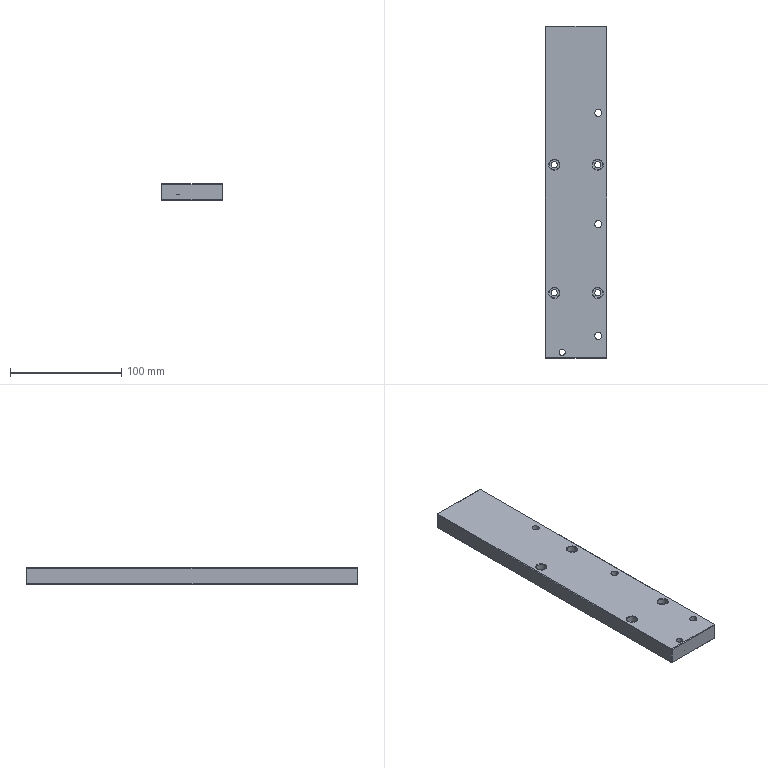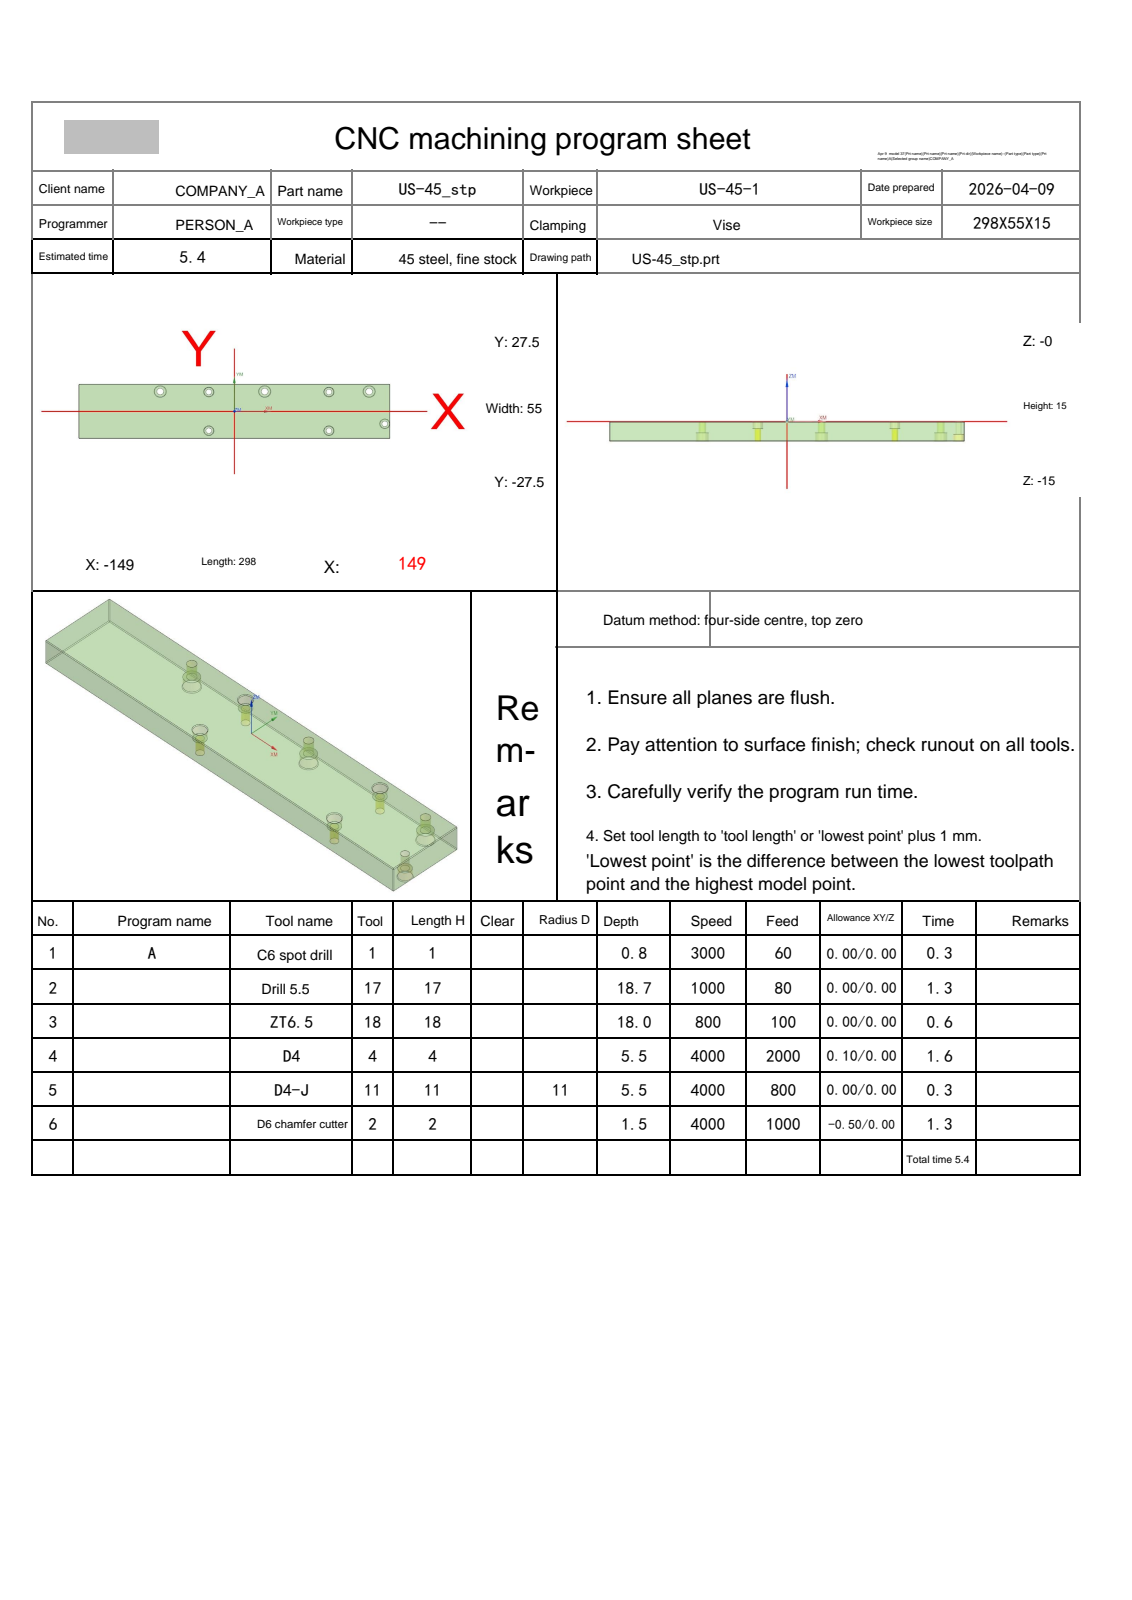NC program | NX | posted by the shop | part box 55 x 298 x 15 mm
Whole program:
%
O0001
(Machine time: 6.47 MIN)
(===Total Tool:6===)
(T1=C6 spot drill   D=6.   R=0.   D-  H01 Z=-0.8  )
(T17=drill 5.5  D=5.5  DR_a=118 D-  H17 Z=-18.65)
(T18=ZT6.5  D=6.5  DR_a=118 D-  H18 Z=-18.  )
(T4=D4      D=4.   R=0.   D-  H04 Z=-5.5  )
(T11=D4-J   D=4.   R=0.   D11 H11 Z=-5.5  )
(T2=D6 chamfer cutter   D=6.   R=0.   D-  H02 Z=-1.5  )
G80 G90 G17 G49 G40
G91 G28 Z0
M01
N1 T01 M06
(C6 spot drill  D=6. R=0. H=01 ce=0.00 di=0.00)
G00 G90 G54 X-71. Y20. M03 S3000
G43 H01 Z20.
M08
G98 G81 X-71. Y20. Z-.8 R1. F60.
X-24.5 Y19.5
Y-19.5
X29. Y20.
X90.5 Y-19.5
Y19.5
X129. Y20.
X144. Y-12.5
G80
G00 Z20.
G91 G28 Z0.0
M05
M09
G91 G28 Z0.0
M01
N2 T17 M06
(drill 5.5 D=5.5 DR_a=118 H=17)
G00 G90 G54 X144. Y-12.5 M03 S1000
G43 H17 Z20.
M08
G98 G83 X144. Y-12.5 Z-18. R1. F80. Q1.
G80
G00 Z20.
G00 G90 X90.5 Y-19.5 M03 S1000
Z20.
G98 G83 X90.5 Y-19.5 Z-18.652 R1. F80. Q1.
Y19.5
X-24.5
Y-19.5
G80
G00 Z20.
G91 G28 Z0.0
M05
M09
G91 G28 Z0.0
M01
N3 T18 M06
(ZT6.5 D=6.5 DR_a=118 H=18)
G00 G90 G54 X-71. Y20. M03 S800
G43 H18 Z20.
M08
G98 G83 X-71. Y20. Z-18. R1. F100. Q1.
X29.
X129.
G80
G00 Z20.
G91 G28 Z0.0
M05
M09
G91 G28 Z0.0
M01
N4 T04 M06
(D4  D=4. R=0. H=04 ce=0.10 di=0.00)
G00 G90 G54 X90.5 Y-19.5 M03 S4000
G43 H04 Z20.
M08
Z1.
G03 X91.1 Y-18.9 I0.0 J.6 F2000.
X90.5 Y-18.3 I-.6 J0.0
X90.5 Y-18.3 Z.8 I0.0 J-1.2
X90.5 Y-18.3 Z.6 I0.0 J-1.2
X90.5 Y-18.3 Z.4 I0.0 J-1.2
X90.5 Y-18.3 Z.2 I0.0 J-1.2
X90.5 Y-18.3 Z0.0 I0.0 J-1.2
X90.5 Y-18.3 Z-.2 I0.0 J-1.2
X90.5 Y-18.3 Z-.4 I0.0 J-1.2
X90.5 Y-18.3 Z-.6 I0.0 J-1.2
X90.5 Y-18.3 Z-.8 I0.0 J-1.2
X90.5 Y-18.3 Z-1. I0.0 J-1.2
X90.5 Y-18.3 Z-1.2 I0.0 J-1.2
X90.5 Y-18.3 Z-1.4 I0.0 J-1.2
X90.5 Y-18.3 Z-1.6 I0.0 J-1.2
X90.5 Y-18.3 Z-1.8 I0.0 J-1.2
X90.5 Y-18.3 Z-2. I0.0 J-1.2
X90.5 Y-18.3 Z-2.2 I0.0 J-1.2
X90.5 Y-18.3 Z-2.4 I0.0 J-1.2
X90.5 Y-18.3 Z-2.6 I0.0 J-1.2
X90.5 Y-18.3 Z-2.8 I0.0 J-1.2
X90.5 Y-18.3 Z-3. I0.0 J-1.2
X90.5 Y-18.3 Z-3.2 I0.0 J-1.2
X90.5 Y-18.3 Z-3.4 I0.0 J-1.2
X90.5 Y-18.3 Z-3.6 I0.0 J-1.2
X90.5 Y-18.3 Z-3.8 I0.0 J-1.2
X90.5 Y-18.3 Z-4. I0.0 J-1.2
X90.5 Y-18.3 Z-4.2 I0.0 J-1.2
X90.5 Y-18.3 Z-4.4 I0.0 J-1.2
X90.5 Y-18.3 Z-4.6 I0.0 J-1.2
X90.5 Y-18.3 Z-4.8 I0.0 J-1.2
X90.5 Y-18.3 Z-5. I0.0 J-1.2
X90.5 Y-18.3 Z-5.2 I0.0 J-1.2
X90.5 Y-18.3 Z-5.4 I0.0 J-1.2
X90.501 Y-20.7 Z-5.5 I0.0 J-1.2
X91.7 Y-19.5 I-.001 J1.2
X90.5 Y-18.3 I-1.2 J0.0
X89.3 Y-19.5 I0.0 J-1.2
X90.5 Y-20.7 I1.2 J0.0
X91.1 Y-20.1 I0.0 J.6
X90.5 Y-19.5 I-.6 J0.0
G00 Z1.
G03 X91.7 Y-18.3 I0.0 J1.2
X90.5 Y-17.1 I-1.2 J0.0
X90.5 Y-17.1 Z.8 I0.0 J-2.4
X90.5 Y-17.1 Z.6 I0.0 J-2.4
X90.5 Y-17.1 Z.4 I0.0 J-2.4
X90.5 Y-17.1 Z.2 I0.0 J-2.4
X90.5 Y-17.1 Z0.0 I0.0 J-2.4
X90.5 Y-17.1 Z-.2 I0.0 J-2.4
X90.5 Y-17.1 Z-.4 I0.0 J-2.4
X90.5 Y-17.1 Z-.6 I0.0 J-2.4
X90.5 Y-17.1 Z-.8 I0.0 J-2.4
X90.5 Y-17.1 Z-1. I0.0 J-2.4
X90.5 Y-17.1 Z-1.2 I0.0 J-2.4
X90.5 Y-17.1 Z-1.4 I0.0 J-2.4
X90.5 Y-17.1 Z-1.6 I0.0 J-2.4
X90.5 Y-17.1 Z-1.8 I0.0 J-2.4
X90.5 Y-17.1 Z-2. I0.0 J-2.4
X90.5 Y-17.1 Z-2.2 I0.0 J-2.4
X90.5 Y-17.1 Z-2.4 I0.0 J-2.4
X90.5 Y-17.1 Z-2.6 I0.0 J-2.4
X90.5 Y-17.1 Z-2.8 I0.0 J-2.4
X90.5 Y-17.1 Z-3. I0.0 J-2.4
X90.5 Y-17.1 Z-3.2 I0.0 J-2.4
X90.5 Y-17.1 Z-3.4 I0.0 J-2.4
X90.5 Y-17.1 Z-3.6 I0.0 J-2.4
X90.5 Y-17.1 Z-3.8 I0.0 J-2.4
X90.5 Y-17.1 Z-4. I0.0 J-2.4
X90.5 Y-17.1 Z-4.2 I0.0 J-2.4
X90.5 Y-17.1 Z-4.4 I0.0 J-2.4
X90.5 Y-17.1 Z-4.6 I0.0 J-2.4
X90.5 Y-17.1 Z-4.8 I0.0 J-2.4
X90.5 Y-17.1 Z-5. I0.0 J-2.4
X90.5 Y-17.1 Z-5.2 I0.0 J-2.4
X90.5 Y-17.1 Z-5.4 I0.0 J-2.4
X90.501 Y-21.9 Z-5.5 I0.0 J-2.4
X92.9 Y-19.5 I-.001 J2.4
X90.5 Y-17.1 I-2.4 J0.0
X88.1 Y-19.5 I0.0 J-2.4
X90.5 Y-21.9 I2.4 J0.0
G01 X90.501
G03 X91.701 Y-20.7 I-.001 J1.2
X90.501 Y-19.5 I-1.2 J0.0
G00 Z20.
X90.5 Y19.5
Z1.
G03 X91.1 Y20.1 I0.0 J.6
X90.5 Y20.7 I-.6 J0.0
X90.5 Y20.7 Z.8 I0.0 J-1.2
X90.5 Y20.7 Z.6 I0.0 J-1.2
X90.5 Y20.7 Z.4 I0.0 J-1.2
X90.5 Y20.7 Z.2 I0.0 J-1.2
X90.5 Y20.7 Z0.0 I0.0 J-1.2
X90.5 Y20.7 Z-.2 I0.0 J-1.2
X90.5 Y20.7 Z-.4 I0.0 J-1.2
X90.5 Y20.7 Z-.6 I0.0 J-1.2
X90.5 Y20.7 Z-.8 I0.0 J-1.2
X90.5 Y20.7 Z-1. I0.0 J-1.2
X90.5 Y20.7 Z-1.2 I0.0 J-1.2
X90.5 Y20.7 Z-1.4 I0.0 J-1.2
X90.5 Y20.7 Z-1.6 I0.0 J-1.2
X90.5 Y20.7 Z-1.8 I0.0 J-1.2
X90.5 Y20.7 Z-2. I0.0 J-1.2
X90.5 Y20.7 Z-2.2 I0.0 J-1.2
X90.5 Y20.7 Z-2.4 I0.0 J-1.2
X90.5 Y20.7 Z-2.6 I0.0 J-1.2
X90.5 Y20.7 Z-2.8 I0.0 J-1.2
X90.5 Y20.7 Z-3. I0.0 J-1.2
X90.5 Y20.7 Z-3.2 I0.0 J-1.2
X90.5 Y20.7 Z-3.4 I0.0 J-1.2
X90.5 Y20.7 Z-3.6 I0.0 J-1.2
X90.5 Y20.7 Z-3.8 I0.0 J-1.2
X90.5 Y20.7 Z-4. I0.0 J-1.2
X90.5 Y20.7 Z-4.2 I0.0 J-1.2
X90.5 Y20.7 Z-4.4 I0.0 J-1.2
X90.5 Y20.7 Z-4.6 I0.0 J-1.2
X90.5 Y20.7 Z-4.8 I0.0 J-1.2
X90.5 Y20.7 Z-5. I0.0 J-1.2
X90.5 Y20.7 Z-5.2 I0.0 J-1.2
X90.5 Y20.7 Z-5.4 I0.0 J-1.2
X90.501 Y18.3 Z-5.5 I0.0 J-1.2
X91.7 Y19.5 I-.001 J1.2
X90.5 Y20.7 I-1.2 J0.0
X89.3 Y19.5 I0.0 J-1.2
X90.5 Y18.3 I1.2 J0.0
X91.1 Y18.9 I0.0 J.6
X90.5 Y19.5 I-.6 J0.0
G00 Z1.
G03 X91.7 Y20.7 I0.0 J1.2
X90.5 Y21.9 I-1.2 J0.0
X90.5 Y21.9 Z.8 I0.0 J-2.4
X90.5 Y21.9 Z.6 I0.0 J-2.4
X90.5 Y21.9 Z.4 I0.0 J-2.4
X90.5 Y21.9 Z.2 I0.0 J-2.4
X90.5 Y21.9 Z0.0 I0.0 J-2.4
X90.5 Y21.9 Z-.2 I0.0 J-2.4
X90.5 Y21.9 Z-.4 I0.0 J-2.4
X90.5 Y21.9 Z-.6 I0.0 J-2.4
X90.5 Y21.9 Z-.8 I0.0 J-2.4
X90.5 Y21.9 Z-1. I0.0 J-2.4
X90.5 Y21.9 Z-1.2 I0.0 J-2.4
X90.5 Y21.9 Z-1.4 I0.0 J-2.4
X90.5 Y21.9 Z-1.6 I0.0 J-2.4
X90.5 Y21.9 Z-1.8 I0.0 J-2.4
X90.5 Y21.9 Z-2. I0.0 J-2.4
X90.5 Y21.9 Z-2.2 I0.0 J-2.4
X90.5 Y21.9 Z-2.4 I0.0 J-2.4
X90.5 Y21.9 Z-2.6 I0.0 J-2.4
X90.5 Y21.9 Z-2.8 I0.0 J-2.4
X90.5 Y21.9 Z-3. I0.0 J-2.4
X90.5 Y21.9 Z-3.2 I0.0 J-2.4
X90.5 Y21.9 Z-3.4 I0.0 J-2.4
X90.5 Y21.9 Z-3.6 I0.0 J-2.4
X90.5 Y21.9 Z-3.8 I0.0 J-2.4
X90.5 Y21.9 Z-4. I0.0 J-2.4
X90.5 Y21.9 Z-4.2 I0.0 J-2.4
X90.5 Y21.9 Z-4.4 I0.0 J-2.4
X90.5 Y21.9 Z-4.6 I0.0 J-2.4
X90.5 Y21.9 Z-4.8 I0.0 J-2.4
X90.5 Y21.9 Z-5. I0.0 J-2.4
X90.5 Y21.9 Z-5.2 I0.0 J-2.4
X90.5 Y21.9 Z-5.4 I0.0 J-2.4
X90.501 Y17.1 Z-5.5 I0.0 J-2.4
X92.9 Y19.5 I-.001 J2.4
X90.5 Y21.9 I-2.4 J0.0
X88.1 Y19.5 I0.0 J-2.4
X90.5 Y17.1 I2.4 J0.0
G01 X90.501
G03 X91.701 Y18.3 I-.001 J1.2
X90.501 Y19.5 I-1.2 J0.0
G00 Z20.
X-24.5
Z1.
G03 X-23.9 Y20.1 I0.0 J.6
X-24.5 Y20.7 I-.6 J0.0
X-24.5 Y20.7 Z.8 I0.0 J-1.2
X-24.5 Y20.7 Z.6 I0.0 J-1.2
X-24.5 Y20.7 Z.4 I0.0 J-1.2
X-24.5 Y20.7 Z.2 I0.0 J-1.2
X-24.5 Y20.7 Z0.0 I0.0 J-1.2
X-24.5 Y20.7 Z-.2 I0.0 J-1.2
X-24.5 Y20.7 Z-.4 I0.0 J-1.2
X-24.5 Y20.7 Z-.6 I0.0 J-1.2
X-24.5 Y20.7 Z-.8 I0.0 J-1.2
X-24.5 Y20.7 Z-1. I0.0 J-1.2
X-24.5 Y20.7 Z-1.2 I0.0 J-1.2
X-24.5 Y20.7 Z-1.4 I0.0 J-1.2
X-24.5 Y20.7 Z-1.6 I0.0 J-1.2
X-24.5 Y20.7 Z-1.8 I0.0 J-1.2
X-24.5 Y20.7 Z-2. I0.0 J-1.2
X-24.5 Y20.7 Z-2.2 I0.0 J-1.2
X-24.5 Y20.7 Z-2.4 I0.0 J-1.2
X-24.5 Y20.7 Z-2.6 I0.0 J-1.2
X-24.5 Y20.7 Z-2.8 I0.0 J-1.2
X-24.5 Y20.7 Z-3. I0.0 J-1.2
X-24.5 Y20.7 Z-3.2 I0.0 J-1.2
X-24.5 Y20.7 Z-3.4 I0.0 J-1.2
X-24.5 Y20.7 Z-3.6 I0.0 J-1.2
X-24.5 Y20.7 Z-3.8 I0.0 J-1.2
X-24.5 Y20.7 Z-4. I0.0 J-1.2
X-24.5 Y20.7 Z-4.2 I0.0 J-1.2
X-24.5 Y20.7 Z-4.4 I0.0 J-1.2
X-24.5 Y20.7 Z-4.6 I0.0 J-1.2
X-24.5 Y20.7 Z-4.8 I0.0 J-1.2
X-24.5 Y20.7 Z-5. I0.0 J-1.2
X-24.5 Y20.7 Z-5.2 I0.0 J-1.2
X-24.5 Y20.7 Z-5.4 I0.0 J-1.2
X-24.499 Y18.3 Z-5.5 I0.0 J-1.2
X-23.3 Y19.5 I-.001 J1.2
X-24.5 Y20.7 I-1.2 J0.0
X-25.7 Y19.5 I0.0 J-1.2
X-24.5 Y18.3 I1.2 J0.0
X-23.9 Y18.9 I0.0 J.6
X-24.5 Y19.5 I-.6 J0.0
G00 Z1.
G03 X-23.3 Y20.7 I0.0 J1.2
X-24.5 Y21.9 I-1.2 J0.0
X-24.5 Y21.9 Z.8 I0.0 J-2.4
X-24.5 Y21.9 Z.6 I0.0 J-2.4
X-24.5 Y21.9 Z.4 I0.0 J-2.4
X-24.5 Y21.9 Z.2 I0.0 J-2.4
X-24.5 Y21.9 Z0.0 I0.0 J-2.4
X-24.5 Y21.9 Z-.2 I0.0 J-2.4
X-24.5 Y21.9 Z-.4 I0.0 J-2.4
X-24.5 Y21.9 Z-.6 I0.0 J-2.4
X-24.5 Y21.9 Z-.8 I0.0 J-2.4
X-24.5 Y21.9 Z-1. I0.0 J-2.4
X-24.5 Y21.9 Z-1.2 I0.0 J-2.4
X-24.5 Y21.9 Z-1.4 I0.0 J-2.4
X-24.5 Y21.9 Z-1.6 I0.0 J-2.4
X-24.5 Y21.9 Z-1.8 I0.0 J-2.4
X-24.5 Y21.9 Z-2. I0.0 J-2.4
X-24.5 Y21.9 Z-2.2 I0.0 J-2.4
X-24.5 Y21.9 Z-2.4 I0.0 J-2.4
X-24.5 Y21.9 Z-2.6 I0.0 J-2.4
X-24.5 Y21.9 Z-2.8 I0.0 J-2.4
X-24.5 Y21.9 Z-3. I0.0 J-2.4
X-24.5 Y21.9 Z-3.2 I0.0 J-2.4
X-24.5 Y21.9 Z-3.4 I0.0 J-2.4
X-24.5 Y21.9 Z-3.6 I0.0 J-2.4
X-24.5 Y21.9 Z-3.8 I0.0 J-2.4
X-24.5 Y21.9 Z-4. I0.0 J-2.4
X-24.5 Y21.9 Z-4.2 I0.0 J-2.4
X-24.5 Y21.9 Z-4.4 I0.0 J-2.4
X-24.5 Y21.9 Z-4.6 I0.0 J-2.4
X-24.5 Y21.9 Z-4.8 I0.0 J-2.4
X-24.5 Y21.9 Z-5. I0.0 J-2.4
X-24.5 Y21.9 Z-5.2 I0.0 J-2.4
X-24.5 Y21.9 Z-5.4 I0.0 J-2.4
X-24.499 Y17.1 Z-5.5 I0.0 J-2.4
X-22.1 Y19.5 I-.001 J2.4
X-24.5 Y21.9 I-2.4 J0.0
X-26.9 Y19.5 I0.0 J-2.4
X-24.5 Y17.1 I2.4 J0.0
G01 X-24.499
G03 X-23.299 Y18.3 I-.001 J1.2
X-24.499 Y19.5 I-1.2 J0.0
G00 Z20.
X-24.5 Y-19.5
Z1.
G03 X-23.9 Y-18.9 I0.0 J.6
X-24.5 Y-18.3 I-.6 J0.0
X-24.5 Y-18.3 Z.8 I0.0 J-1.2
X-24.5 Y-18.3 Z.6 I0.0 J-1.2
X-24.5 Y-18.3 Z.4 I0.0 J-1.2
X-24.5 Y-18.3 Z.2 I0.0 J-1.2
X-24.5 Y-18.3 Z0.0 I0.0 J-1.2
X-24.5 Y-18.3 Z-.2 I0.0 J-1.2
X-24.5 Y-18.3 Z-.4 I0.0 J-1.2
X-24.5 Y-18.3 Z-.6 I0.0 J-1.2
X-24.5 Y-18.3 Z-.8 I0.0 J-1.2
X-24.5 Y-18.3 Z-1. I0.0 J-1.2
X-24.5 Y-18.3 Z-1.2 I0.0 J-1.2
X-24.5 Y-18.3 Z-1.4 I0.0 J-1.2
X-24.5 Y-18.3 Z-1.6 I0.0 J-1.2
X-24.5 Y-18.3 Z-1.8 I0.0 J-1.2
X-24.5 Y-18.3 Z-2. I0.0 J-1.2
X-24.5 Y-18.3 Z-2.2 I0.0 J-1.2
X-24.5 Y-18.3 Z-2.4 I0.0 J-1.2
X-24.5 Y-18.3 Z-2.6 I0.0 J-1.2
X-24.5 Y-18.3 Z-2.8 I0.0 J-1.2
X-24.5 Y-18.3 Z-3. I0.0 J-1.2
X-24.5 Y-18.3 Z-3.2 I0.0 J-1.2
X-24.5 Y-18.3 Z-3.4 I0.0 J-1.2
X-24.5 Y-18.3 Z-3.6 I0.0 J-1.2
X-24.5 Y-18.3 Z-3.8 I0.0 J-1.2
X-24.5 Y-18.3 Z-4. I0.0 J-1.2
X-24.5 Y-18.3 Z-4.2 I0.0 J-1.2
X-24.5 Y-18.3 Z-4.4 I0.0 J-1.2
X-24.5 Y-18.3 Z-4.6 I0.0 J-1.2
X-24.5 Y-18.3 Z-4.8 I0.0 J-1.2
X-24.5 Y-18.3 Z-5. I0.0 J-1.2
X-24.5 Y-18.3 Z-5.2 I0.0 J-1.2
X-24.5 Y-18.3 Z-5.4 I0.0 J-1.2
X-24.499 Y-20.7 Z-5.5 I0.0 J-1.2
X-23.3 Y-19.5 I-.001 J1.2
X-24.5 Y-18.3 I-1.2 J0.0
X-25.7 Y-19.5 I0.0 J-1.2
X-24.5 Y-20.7 I1.2 J0.0
X-23.9 Y-20.1 I0.0 J.6
X-24.5 Y-19.5 I-.6 J0.0
G00 Z1.
G03 X-23.3 Y-18.3 I0.0 J1.2
X-24.5 Y-17.1 I-1.2 J0.0
X-24.5 Y-17.1 Z.8 I0.0 J-2.4
X-24.5 Y-17.1 Z.6 I0.0 J-2.4
X-24.5 Y-17.1 Z.4 I0.0 J-2.4
X-24.5 Y-17.1 Z.2 I0.0 J-2.4
X-24.5 Y-17.1 Z0.0 I0.0 J-2.4
X-24.5 Y-17.1 Z-.2 I0.0 J-2.4
X-24.5 Y-17.1 Z-.4 I0.0 J-2.4
X-24.5 Y-17.1 Z-.6 I0.0 J-2.4
X-24.5 Y-17.1 Z-.8 I0.0 J-2.4
X-24.5 Y-17.1 Z-1. I0.0 J-2.4
X-24.5 Y-17.1 Z-1.2 I0.0 J-2.4
X-24.5 Y-17.1 Z-1.4 I0.0 J-2.4
X-24.5 Y-17.1 Z-1.6 I0.0 J-2.4
X-24.5 Y-17.1 Z-1.8 I0.0 J-2.4
X-24.5 Y-17.1 Z-2. I0.0 J-2.4
X-24.5 Y-17.1 Z-2.2 I0.0 J-2.4
X-24.5 Y-17.1 Z-2.4 I0.0 J-2.4
X-24.5 Y-17.1 Z-2.6 I0.0 J-2.4
X-24.5 Y-17.1 Z-2.8 I0.0 J-2.4
X-24.5 Y-17.1 Z-3. I0.0 J-2.4
X-24.5 Y-17.1 Z-3.2 I0.0 J-2.4
X-24.5 Y-17.1 Z-3.4 I0.0 J-2.4
X-24.5 Y-17.1 Z-3.6 I0.0 J-2.4
X-24.5 Y-17.1 Z-3.8 I0.0 J-2.4
X-24.5 Y-17.1 Z-4. I0.0 J-2.4
X-24.5 Y-17.1 Z-4.2 I0.0 J-2.4
X-24.5 Y-17.1 Z-4.4 I0.0 J-2.4
X-24.5 Y-17.1 Z-4.6 I0.0 J-2.4
X-24.5 Y-17.1 Z-4.8 I0.0 J-2.4
X-24.5 Y-17.1 Z-5. I0.0 J-2.4
X-24.5 Y-17.1 Z-5.2 I0.0 J-2.4
X-24.5 Y-17.1 Z-5.4 I0.0 J-2.4
X-24.499 Y-21.9 Z-5.5 I0.0 J-2.4
X-22.1 Y-19.5 I-.001 J2.4
X-24.5 Y-17.1 I-2.4 J0.0
X-26.9 Y-19.5 I0.0 J-2.4
X-24.5 Y-21.9 I2.4 J0.0
G01 X-24.499
G03 X-23.299 Y-20.7 I-.001 J1.2
X-24.499 Y-19.5 I-1.2 J0.0
G00 Z20.
G91 G28 Z0.0
M05
M09
G91 G28 Z0.0
M01
N5 T11 M06
(D4-J  D=4. R=0. H=11 ce=0.00 di=0.00)
G00 G90 G54 X90.5 Y-19.5 M03 S4000
G43 H11 Z20.
M08
Z1.
G41 D11
G01 X90.697 Y-19.468 F800.
G03 X91.742 Y-18.242 I-.197 J1.226
X90.5 Y-17. I-1.242 J0.0
X90.5 Y-17. Z-4. I0.0 J-2.5
X88.122 Y-20.273 Z-5.5 I0.0 J-2.5
X90.5 Y-22. I2.378 J.773
X93. Y-19.5 I0.0 J2.5
X90.5 Y-17. I-2.5 J0.0
X88. Y-19.5 I0.0 J-2.5
X88.122 Y-20.273 I2.5 J0.0
X89.304 Y-21.131 I1.181 J.384
X90.546 Y-19.889 I0.0 J1.242
G01 X90.531 Y-19.698
G40 X90.5 Y-19.5
G00 Z20.
Y19.5
Z1.
G41 D11
G01 X90.697 Y19.532
G03 X91.742 Y20.758 I-.197 J1.226
X90.5 Y22. I-1.242 J0.0
X90.5 Y22. Z-4. I0.0 J-2.5
X88.122 Y18.727 Z-5.5 I0.0 J-2.5
X90.5 Y17. I2.378 J.773
X93. Y19.5 I0.0 J2.5
X90.5 Y22. I-2.5 J0.0
X88. Y19.5 I0.0 J-2.5
X88.122 Y18.727 I2.5 J0.0
X89.304 Y17.869 I1.181 J.384
X90.546 Y19.111 I0.0 J1.242
G01 X90.531 Y19.302
G40 X90.5 Y19.5
G00 Z20.
X-24.5
Z1.
G41 D11
G01 X-24.303 Y19.532
G03 X-23.258 Y20.758 I-.197 J1.226
X-24.5 Y22. I-1.242 J0.0
X-24.5 Y22. Z-4. I0.0 J-2.5
X-26.878 Y18.727 Z-5.5 I0.0 J-2.5
X-24.5 Y17. I2.378 J.773
X-22. Y19.5 I0.0 J2.5
X-24.5 Y22. I-2.5 J0.0
X-27. Y19.5 I0.0 J-2.5
X-26.878 Y18.727 I2.5 J0.0
X-25.696 Y17.869 I1.181 J.384
X-24.454 Y19.111 I0.0 J1.242
G01 X-24.469 Y19.302
G40 X-24.5 Y19.5
G00 Z20.
Y-19.5
Z1.
G41 D11
G01 X-24.303 Y-19.468
G03 X-23.258 Y-18.242 I-.197 J1.226
X-24.5 Y-17. I-1.242 J0.0
X-24.5 Y-17. Z-4. I0.0 J-2.5
X-26.878 Y-20.273 Z-5.5 I0.0 J-2.5
X-24.5 Y-22. I2.378 J.773
X-22. Y-19.5 I0.0 J2.5
X-24.5 Y-17. I-2.5 J0.0
X-27. Y-19.5 I0.0 J-2.5
X-26.878 Y-20.273 I2.5 J0.0
X-25.696 Y-21.131 I1.181 J.384
X-24.454 Y-19.889 I0.0 J1.242
G01 X-24.469 Y-19.698
G40 X-24.5 Y-19.5
G00 Z20.
G91 G28 Z0.0
M05
M09
G91 G28 Z0.0
M01
N6 T02 M06
(D6 chamfer cutter  D=6. R=0. H=02 ce=-0.30 di=0.00)
G00 G90 G54 X145.118 Y-11.941 M03 S4000
G43 H02 Z20.
M08
Z-.3
G01 Z-.8 F300.
X145.5 Y-11.75
G03 X144. Y-10.25 I-1.5 J0.0
X141.75 Y-12.5 I0.0 J-2.25
X144. Y-14.75 I2.25 J0.0
X146.25 Y-12.5 I0.0 J2.25
X144. Y-10.25 I-2.25 J0.0
X142.5 Y-11.75 I0.0 J-1.5
G01 X142.882 Y-11.941
Z-.3
G00 Z20.
G00 G90 X130.5 Y20.391 M03 S4000
Z20.
Z-.5
G01 Z-1. F400.
Y21.05
G03 X129. Y22.55 I-1.5 J0.0
X126.45 Y20. I0.0 J-2.55
X129. Y17.45 I2.55 J0.0
X131.55 Y20. I0.0 J2.55
X129. Y22.55 I-2.55 J0.0
X127.5 Y21.05 I0.0 J-1.5
G01 Y20.391
Z-.5
G00 Z20.
X30.5
Z-.5
G01 Z-1.
Y21.05
G03 X29. Y22.55 I-1.5 J0.0
X26.45 Y20. I0.0 J-2.55
X29. Y17.45 I2.55 J0.0
X31.55 Y20. I0.0 J2.55
X29. Y22.55 I-2.55 J0.0
X27.5 Y21.05 I0.0 J-1.5
G01 Y20.391
Z-.5
G00 Z20.
X-69.5
Z-.5
G01 Z-1.
Y21.05
G03 X-71. Y22.55 I-1.5 J0.0
X-73.55 Y20. I0.0 J-2.55
X-71. Y17.45 I2.55 J0.0
X-68.45 Y20. I0.0 J2.55
X-71. Y22.55 I-2.55 J0.0
X-72.5 Y21.05 I0.0 J-1.5
G01 Y20.391
Z-.5
G00 Z20.
G00 G90 X90.509 Y15.998 M03 S4000
Z20.
Z2.5
G01 X90.891 Y16.019 Z2.361 F500.
X91.276 Y16.084 Z2.219
X91.653 Y16.192 Z2.076
X92.014 Y16.341 Z1.934
X92.357 Y16.53 Z1.791
X92.677 Y16.755 Z1.649
X92.969 Y17.015 Z1.507
X93.231 Y17.306 Z1.364
X93.459 Y17.624 Z1.222
X93.604 Y17.876 Z1.116
X93.765 Y18.232 Z.974
X93.886 Y18.604 Z.831
X93.965 Y18.987 Z.689
X94.001 Y19.377 Z.547
X93.993 Y19.768 Z.404
X93.941 Y20.156 Z.262
X93.846 Y20.535 Z.119
X93.71 Y20.902 Z-.023
X93.534 Y21.252 Z-.166
X93.319 Y21.579 Z-.308
X93.07 Y21.88 Z-.45
X92.788 Y22.152 Z-.593
X92.478 Y22.391 Z-.735
X92.144 Y22.593 Z-.878
X91.788 Y22.757 Z-1.02
X91.417 Y22.881 Z-1.162
X91.034 Y22.962 Z-1.305
X90.645 Y23. Z-1.447
X90.5 Z-1.5
G03 X87. Y19.5 I0.0 J-3.5
X90.5 Y16. I3.5 J0.0
X94. Y19.5 I0.0 J3.5
X90.5 Y23. I-3.5 J0.0
X90.002 Y22.964 I0.0 J-3.5
G01 Z1.
G00 Z20.
X90.509 Y-23.002
Z2.5
G01 X90.891 Y-22.981 Z2.361
X91.276 Y-22.916 Z2.219
X91.653 Y-22.808 Z2.076
X92.014 Y-22.659 Z1.934
X92.357 Y-22.47 Z1.791
X92.677 Y-22.245 Z1.649
X92.969 Y-21.985 Z1.507
X93.231 Y-21.694 Z1.364
X93.459 Y-21.376 Z1.222
X93.604 Y-21.124 Z1.116
X93.765 Y-20.768 Z.974
X93.886 Y-20.396 Z.831
X93.965 Y-20.013 Z.689
X94.001 Y-19.623 Z.547
X93.993 Y-19.232 Z.404
X93.941 Y-18.844 Z.262
X93.846 Y-18.465 Z.119
X93.71 Y-18.098 Z-.023
X93.534 Y-17.749 Z-.166
X93.319 Y-17.421 Z-.308
X93.07 Y-17.12 Z-.45
X92.788 Y-16.848 Z-.593
X92.478 Y-16.609 Z-.735
X92.144 Y-16.407 Z-.878
X91.788 Y-16.243 Z-1.02
X91.417 Y-16.119 Z-1.162
X91.034 Y-16.038 Z-1.305
X90.645 Y-16. Z-1.447
X90.5 Z-1.5
G03 X87. Y-19.5 I0.0 J-3.5
X90.5 Y-23. I3.5 J0.0
X94. Y-19.5 I0.0 J3.5
X90.5 Y-16. I-3.5 J0.0
X90.002 Y-16.036 I0.0 J-3.5
G01 Z1.
G00 Z20.
X-24.491 Y-23.002
Z2.5
G01 X-24.109 Y-22.981 Z2.361
X-23.724 Y-22.916 Z2.219
X-23.347 Y-22.808 Z2.076
X-22.986 Y-22.659 Z1.934
X-22.643 Y-22.47 Z1.791
X-22.323 Y-22.245 Z1.649
X-22.031 Y-21.985 Z1.507
X-21.769 Y-21.694 Z1.364
X-21.541 Y-21.376 Z1.222
X-21.396 Y-21.124 Z1.116
X-21.235 Y-20.768 Z.974
X-21.114 Y-20.396 Z.831
X-21.035 Y-20.013 Z.689
X-20.999 Y-19.623 Z.547
X-21.007 Y-19.232 Z.404
X-21.059 Y-18.844 Z.262
X-21.154 Y-18.465 Z.119
X-21.29 Y-18.098 Z-.023
X-21.466 Y-17.749 Z-.166
X-21.681 Y-17.421 Z-.308
X-21.93 Y-17.12 Z-.45
X-22.212 Y-16.848 Z-.593
X-22.522 Y-16.609 Z-.735
X-22.856 Y-16.407 Z-.878
X-23.212 Y-16.243 Z-1.02
X-23.583 Y-16.119 Z-1.162
X-23.966 Y-16.038 Z-1.305
X-24.355 Y-16. Z-1.447
X-24.5 Z-1.5
G03 X-28. Y-19.5 I0.0 J-3.5
X-24.5 Y-23. I3.5 J0.0
X-21. Y-19.5 I0.0 J3.5
X-24.5 Y-16. I-3.5 J0.0
X-24.998 Y-16.036 I0.0 J-3.5
G01 Z1.
G00 Z20.
X-24.491 Y15.998
Z2.5
G01 X-24.109 Y16.019 Z2.361
X-23.724 Y16.084 Z2.219
X-23.347 Y16.192 Z2.076
X-22.986 Y16.341 Z1.934
X-22.643 Y16.53 Z1.791
X-22.323 Y16.755 Z1.649
X-22.031 Y17.015 Z1.507
X-21.769 Y17.306 Z1.364
X-21.541 Y17.624 Z1.222
X-21.396 Y17.876 Z1.116
X-21.235 Y18.232 Z.974
X-21.114 Y18.604 Z.831
X-21.035 Y18.987 Z.689
X-20.999 Y19.377 Z.547
X-21.007 Y19.768 Z.404
X-21.059 Y20.156 Z.262
X-21.154 Y20.535 Z.119
X-21.29 Y20.902 Z-.023
X-21.466 Y21.252 Z-.166
X-21.681 Y21.579 Z-.308
X-21.93 Y21.88 Z-.45
X-22.212 Y22.152 Z-.593
X-22.522 Y22.391 Z-.735
X-22.856 Y22.593 Z-.878
X-23.212 Y22.757 Z-1.02
X-23.583 Y22.881 Z-1.162
X-23.966 Y22.962 Z-1.305
X-24.355 Y23. Z-1.447
X-24.5 Z-1.5
G03 X-28. Y19.5 I0.0 J-3.5
X-24.5 Y16. I3.5 J0.0
X-21. Y19.5 I0.0 J3.5
X-24.5 Y23. I-3.5 J0.0
X-24.998 Y22.964 I0.0 J-3.5
G01 Z1.
G00 Z20.
G00 G90 X-139.869 Y-28.5 M03 S4000
Z20.
Z2.5
G01 X-148.5 Z-.642 F1000.
X-148.595 Z-.676
X-148.833 Y-28.466 Z-.764
X-149.063 Y-28.393 Z-.852
X-149.279 Y-28.286 Z-.939
X-149.474 Y-28.145 Z-1.027
X-149.645 Y-27.974 Z-1.115
X-149.786 Y-27.779 Z-1.202
X-149.893 Y-27.563 Z-1.29
X-149.966 Y-27.333 Z-1.378
X-150. Y-27.095 Z-1.465
Y-27. Z-1.5
Y27.
G02 X-148.5 Y28.5 I1.5 J0.0
G01 X148.5
G02 X150. Y27. I0.0 J-1.5
G01 Y-27.
G02 X148.5 Y-28.5 I-1.5 J0.0
G01 X-148.5
G02 X-150. Y-27. I0.0 J1.5
G01 Y-26.5
Z1.
G00 Z20.
M05
M09
G91 G28 Z0.0
G91 G28 Y0.0
M30
%